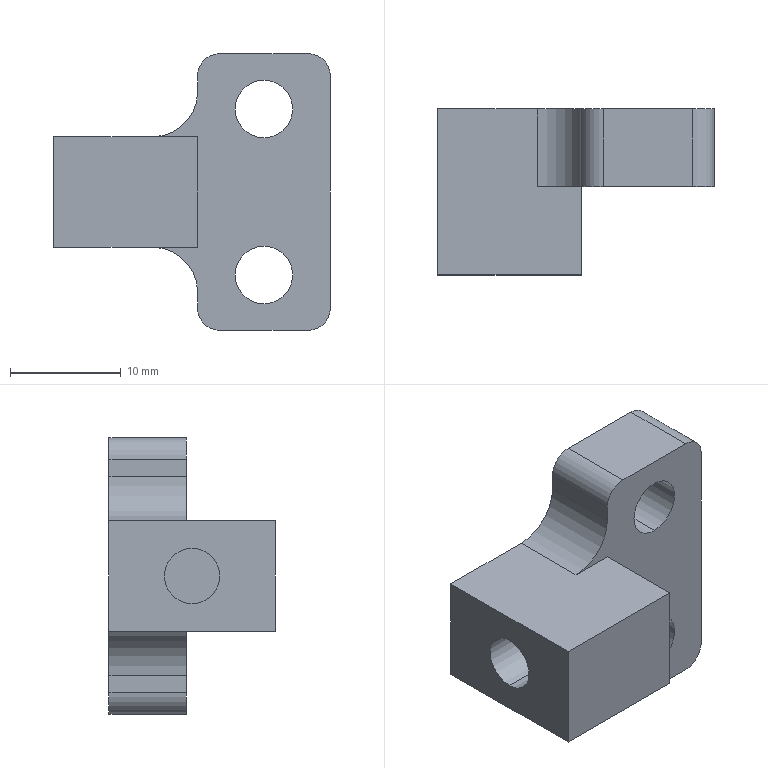NC program | Mastercam | posted with a generic post
Lines 16711 to 16956 of 16956:
N8730 T6 M6
N8740 G0 G90 G17 G54 X-15.5 Y-12.687 A0. S7000 M3
N8750 G43 H6 Z50. M8
N8760 Z1.
N8770 G1 Z-8. F600.
N8780 Y-.687 F1000.
N8790 Y5.
N8800 G2 X-12.5 Y8. I3. J0.
N8810 G1 X.5
N8820 G2 X3.5 Y5. I0. J-3.
N8830 G1 Y-5.
N8840 G2 X.5 Y-8. I-3. J0.
N8850 G1 X-12.5
N8860 G2 X-15.5 Y-5. I0. J3.
N8870 G1 Y-.687
N8880 Y11.313
N8890 G0 Z50.
N8900 X10.306 Y15.5
N8910 Z-7.
N8920 G1 Z-8. F600.
N8930 G2 X13.098 Y11.948 I-10.957 J-11.484 F500.
N8940 X14.693 Y7.365 I-17.281 J-8.586
N8950 X14.907 Y1.454 I-81.513 J-5.911
N8960 X14.894 Y0. I-81.727 J0.
N8970 X14.98 Y-2.56 I-38.033 J-2.56
N8980 X14.631 Y-7.711 I-38.119 J0.
N8990 X12.294 Y-13.249 I-15.866 J3.433
N9000 X10.287 Y-15.5 I-13.257 J9.797
N9010 G0 Z50.
N9020 X3.303 Y15.5
N9030 Z-7.
N9040 G1 Z-8. F600.
N9050 G2 X9.064 Y11.704 I-2.873 J-10.629 F500.
N9060 X11.172 Y7.087 I-9.943 J-7.331
N9070 X11.48 Y2.575 I-32.938 J-4.512
N9080 X11.38 Y0. I-33.246 J0.
N9090 X11.48 Y-2.575 I-33.146 J-2.575
N9100 X11.172 Y-7.087 I-33.246 J0.
N9110 X9.064 Y-11.704 I-12.051 J2.714
N9120 X3.303 Y-15.5 I-8.634 J6.833
N9130 G0 Z50.
N9140 X-1.806 Y13.037
N9150 Z-7.
N9160 G1 Z-8. F600.
N9170 X-.751 Y12.071 F500.
N9180 X.246
N9190 G2 X.432 Y12.073 I.186 J-7.174
N9200 X6.499 Y8.73 I0. J-7.176
N9210 X7.486 Y6.064 I-8.051 J-4.496
N9220 G1 X7.571 Y0.
N9230 G2 X7.667 Y-2.557 I-34.068 J-2.557
N9240 X7.486 Y-6.064 I-34.164 J0.
N9250 X5.881 Y-9.582 I-8.168 J1.601
N9260 X.169 Y-12.126 I-5.712 J5.14
N9270 X-.751 Y-12.071 I0. J7.684
N9280 G1 X-1.806 Y-13.037
N9290 G0 Z50.
N9300 X-2.673 Y8.447
N9310 Z-7.
N9320 G1 Z-8. F600.
N9330 X-2.295 Y8.1 F500.
N9340 X.245
N9350 G2 X.438 Y8.106 I.193 J-3.261
N9360 X1.974 Y7.723 I0. J-3.267
N9370 X3.356 Y6.186 I-1.411 J-2.66
N9380 X3.6 Y5.013 I-2.853 J-1.205
N9390 G1 Y0.
N9400 Y-5.013
N9410 X3.578 Y-5.359
N9420 G2 X2.791 Y-7.088 I-3.21 J.418
N9430 X.937 Y-8.068 I-2.33 J2.165
N9440 G1 X.591 Y-8.099
N9450 X-2.295 Y-8.1
N9460 X-2.673 Y-8.447
N9470 G0 Z50.
N9480 X-2.732 Y-13.881
N9490 Z1.
N9500 G1 Z-15.5 F600.
N9510 X-2.199 Y-13.605 F1000.
N9520 G3 X-1.874 Y-13.072 I-.275 J.533
N9530 X-1.941 Y-12.797 I-.6 J0.
N9540 G2 X-2.5 Y-10.5 I4.441 J2.297
N9550 G1 Y-9.
N9560 G3 X-3.5 Y-8. I-1. J0.
N9570 G1 X-12.5
N9580 G2 X-15.5 Y-5. I0. J3.
N9590 G1 Y5.
N9600 G2 X-12.5 Y8. I3. J0.
N9610 G1 X-3.5
N9620 G3 X-2.5 Y9. I0. J1.
N9630 G1 Y10.5
N9640 G2 X2.5 Y15.5 I5. J0.
N9650 G1 X10.5
N9660 G2 X15.5 Y10.5 I0. J-5.
N9670 G1 Y-10.5
N9680 G2 X10.5 Y-15.5 I-5. J0.
N9690 G1 X2.5
N9700 G2 X-1.941 Y-12.797 I0. J5.
N9710 G3 X-2.474 Y-12.472 I-.533 J-.275
N9720 X-2.75 Y-12.539 I0. J-.6
N9730 G1 X-3.283 Y-12.815
N9740 G0 Z50.
N9750 X-2.732 Y-13.881
N9760 Z1.
N9770 G1 Z-15.5 F600.
N9780 X-2.199 Y-13.605 F1000.
N9790 G3 X-1.874 Y-13.072 I-.275 J.533
N9800 X-1.941 Y-12.797 I-.6 J0.
N9810 G2 X-2.5 Y-10.5 I4.441 J2.297
N9820 G1 Y-9.
N9830 G3 X-3.5 Y-8. I-1. J0.
N9840 G1 X-12.5
N9850 G2 X-15.5 Y-5. I0. J3.
N9860 G1 Y5.
N9870 G2 X-12.5 Y8. I3. J0.
N9880 G1 X-3.5
N9890 G3 X-2.5 Y9. I0. J1.
N9900 G1 Y10.5
N9910 G2 X2.5 Y15.5 I5. J0.
N9920 G1 X10.5
N9930 G2 X15.5 Y10.5 I0. J-5.
N9940 G1 Y-10.5
N9950 G2 X10.5 Y-15.5 I-5. J0.
N9960 G1 X2.5
N9970 G2 X-1.941 Y-12.797 I0. J5.
N9980 G3 X-2.474 Y-12.472 I-.533 J-.275
N9990 X-2.75 Y-12.539 I0. J-.6
N100 G1 X-3.283 Y-12.815
N110 G0 Z50.
N120 M5
N130 G91 G28 Z0. M9
N140 A0.
N150 M01
N160 T7 M6
N170 G0 G90 G17 G54 X6.5 Y7.5 A0. S3000 M3
N180 G43 H7 Z42. M8
N190 G98 G81 Z-8.7 R-7. F300.
N200 Y-7.5
N210 G80
N220 S7000 M3
N230 G0 X3.15 Y6. Z25.3
N240 Z.3
N250 G1 Z-.7 F1000.
N260 X2.15
N270 G3 X1.15 Y5. I0. J-1.
N280 G1 Y-5.
N290 G2 X.5 Y-5.65 I-.65 J0.
N300 G1 X-12.5
N310 G2 X-13.15 Y-5. I0. J.65
N320 G1 Y5.
N330 G2 X-12.5 Y5.65 I.65 J0.
N340 G1 X.5
N350 G2 X1.15 Y5. I0. J-.65
N360 G3 X2.15 Y4. I1. J0.
N370 G1 X3.15
N380 G0 Z24.3
N390 Z24.989
N400 X-2.545 Y7.618
N410 Z17.3
N420 Z-7.7
N430 G1 Z-8.7 F1000.
N440 X-1.598 Y7.295
N450 G3 X-1.276 Y7.242 I.322 J.947
N460 X-.329 Y7.919 I0. J1.
N470 X-.15 Y9. I-3.171 J1.081
N480 G1 Y10.5
N490 G2 X2.5 Y13.15 I2.65 J0.
N500 G1 X10.5
N510 G2 X13.15 Y10.5 I0. J-2.65
N520 G1 Y-10.5
N530 G2 X10.5 Y-13.15 I-2.65 J0.
N540 G1 X2.5
N550 G2 X-.15 Y-10.5 I0. J2.65
N560 G1 Y-9.
N570 G3 X-.329 Y-7.919 I-3.35 J0.
N580 X-1.276 Y-7.241 I-.947 J-.323
N590 X-1.598 Y-7.295 I0. J-1.001
N600 G1 X-2.545 Y-7.618
N610 G0 Z16.3
N620 Z24.857
N630 M5
N640 G91 G28 Z0. M9
N650 A0.
N660 M01
N670 T24 M6
N680 G0 G90 G17 G54 X0. Y-86.8 A0. S4000 M3
N690 G43 H24 Z55. M8
N700 Z7.
N710 G1 Z4.51 F600.
N720 Y86.8 F3000.
N730 Z4.02 F600.
N740 Y-86.8 F3000.
N750 Z3.53 F600.
N760 Y86.8 F3000.
N770 Z3.04 F600.
N780 Y-86.8 F3000.
N790 Z2.55 F600.
N800 Y86.8 F3000.
N810 Z2.06 F600.
N820 Y-86.8 F3000.
N830 Z1.57 F600.
N840 Y86.8 F3000.
N850 Z1.08 F600.
N860 Y-86.8 F3000.
N870 Z.59 F600.
N880 Y86.8 F3000.
N890 Z.1 F600.
N900 Y-86.8 F3000.
N910 Z0. F600.
N920 Y86.8 F1000.
N930 G0 Z50.
N940 M5
N950 G91 G28 Z0. M9
N960 A0.
N970 M01
N980 T7 M6
N990 G0 G90 G17 G54 X-5.4 Y13.95 A0. S7000 M3
N1000 G43 H7 Z50. M8
N1010 Z1.
N1020 G1 Z-.8 F600.
N1030 Y13.55 F1000.
N1040 G3 X-5. Y13.15 I.4 J0.
N1050 G1 X5.
N1060 G2 X5.65 Y12.5 I0. J-.65
N1070 G1 Y3.5
N1080 G3 X9. Y.15 I3.35 J0.
N1090 G1 X10.5
N1100 G2 X13.15 Y-2.5 I0. J-2.65
N1110 G1 Y-10.5
N1120 G2 X10.5 Y-13.15 I-2.65 J0.
N1130 G1 X-10.5
N1140 G2 X-13.15 Y-10.5 I0. J2.65
N1150 G1 Y-2.5
N1160 G2 X-10.5 Y.15 I2.65 J0.
N1170 G1 X-9.
N1180 G3 X-5.65 Y3.5 I0. J3.35
N1190 G1 Y12.5
N1200 G2 X-5. Y13.15 I.65 J0.
N1210 G3 X-4.6 Y13.55 I0. J.4
N1220 G1 Y13.95
N1230 G0 Z50.
N1240 M5
N1250 G91 G28 Z0. M9
N1260 G28 X0. Y0. A0.
N1270 M30
%